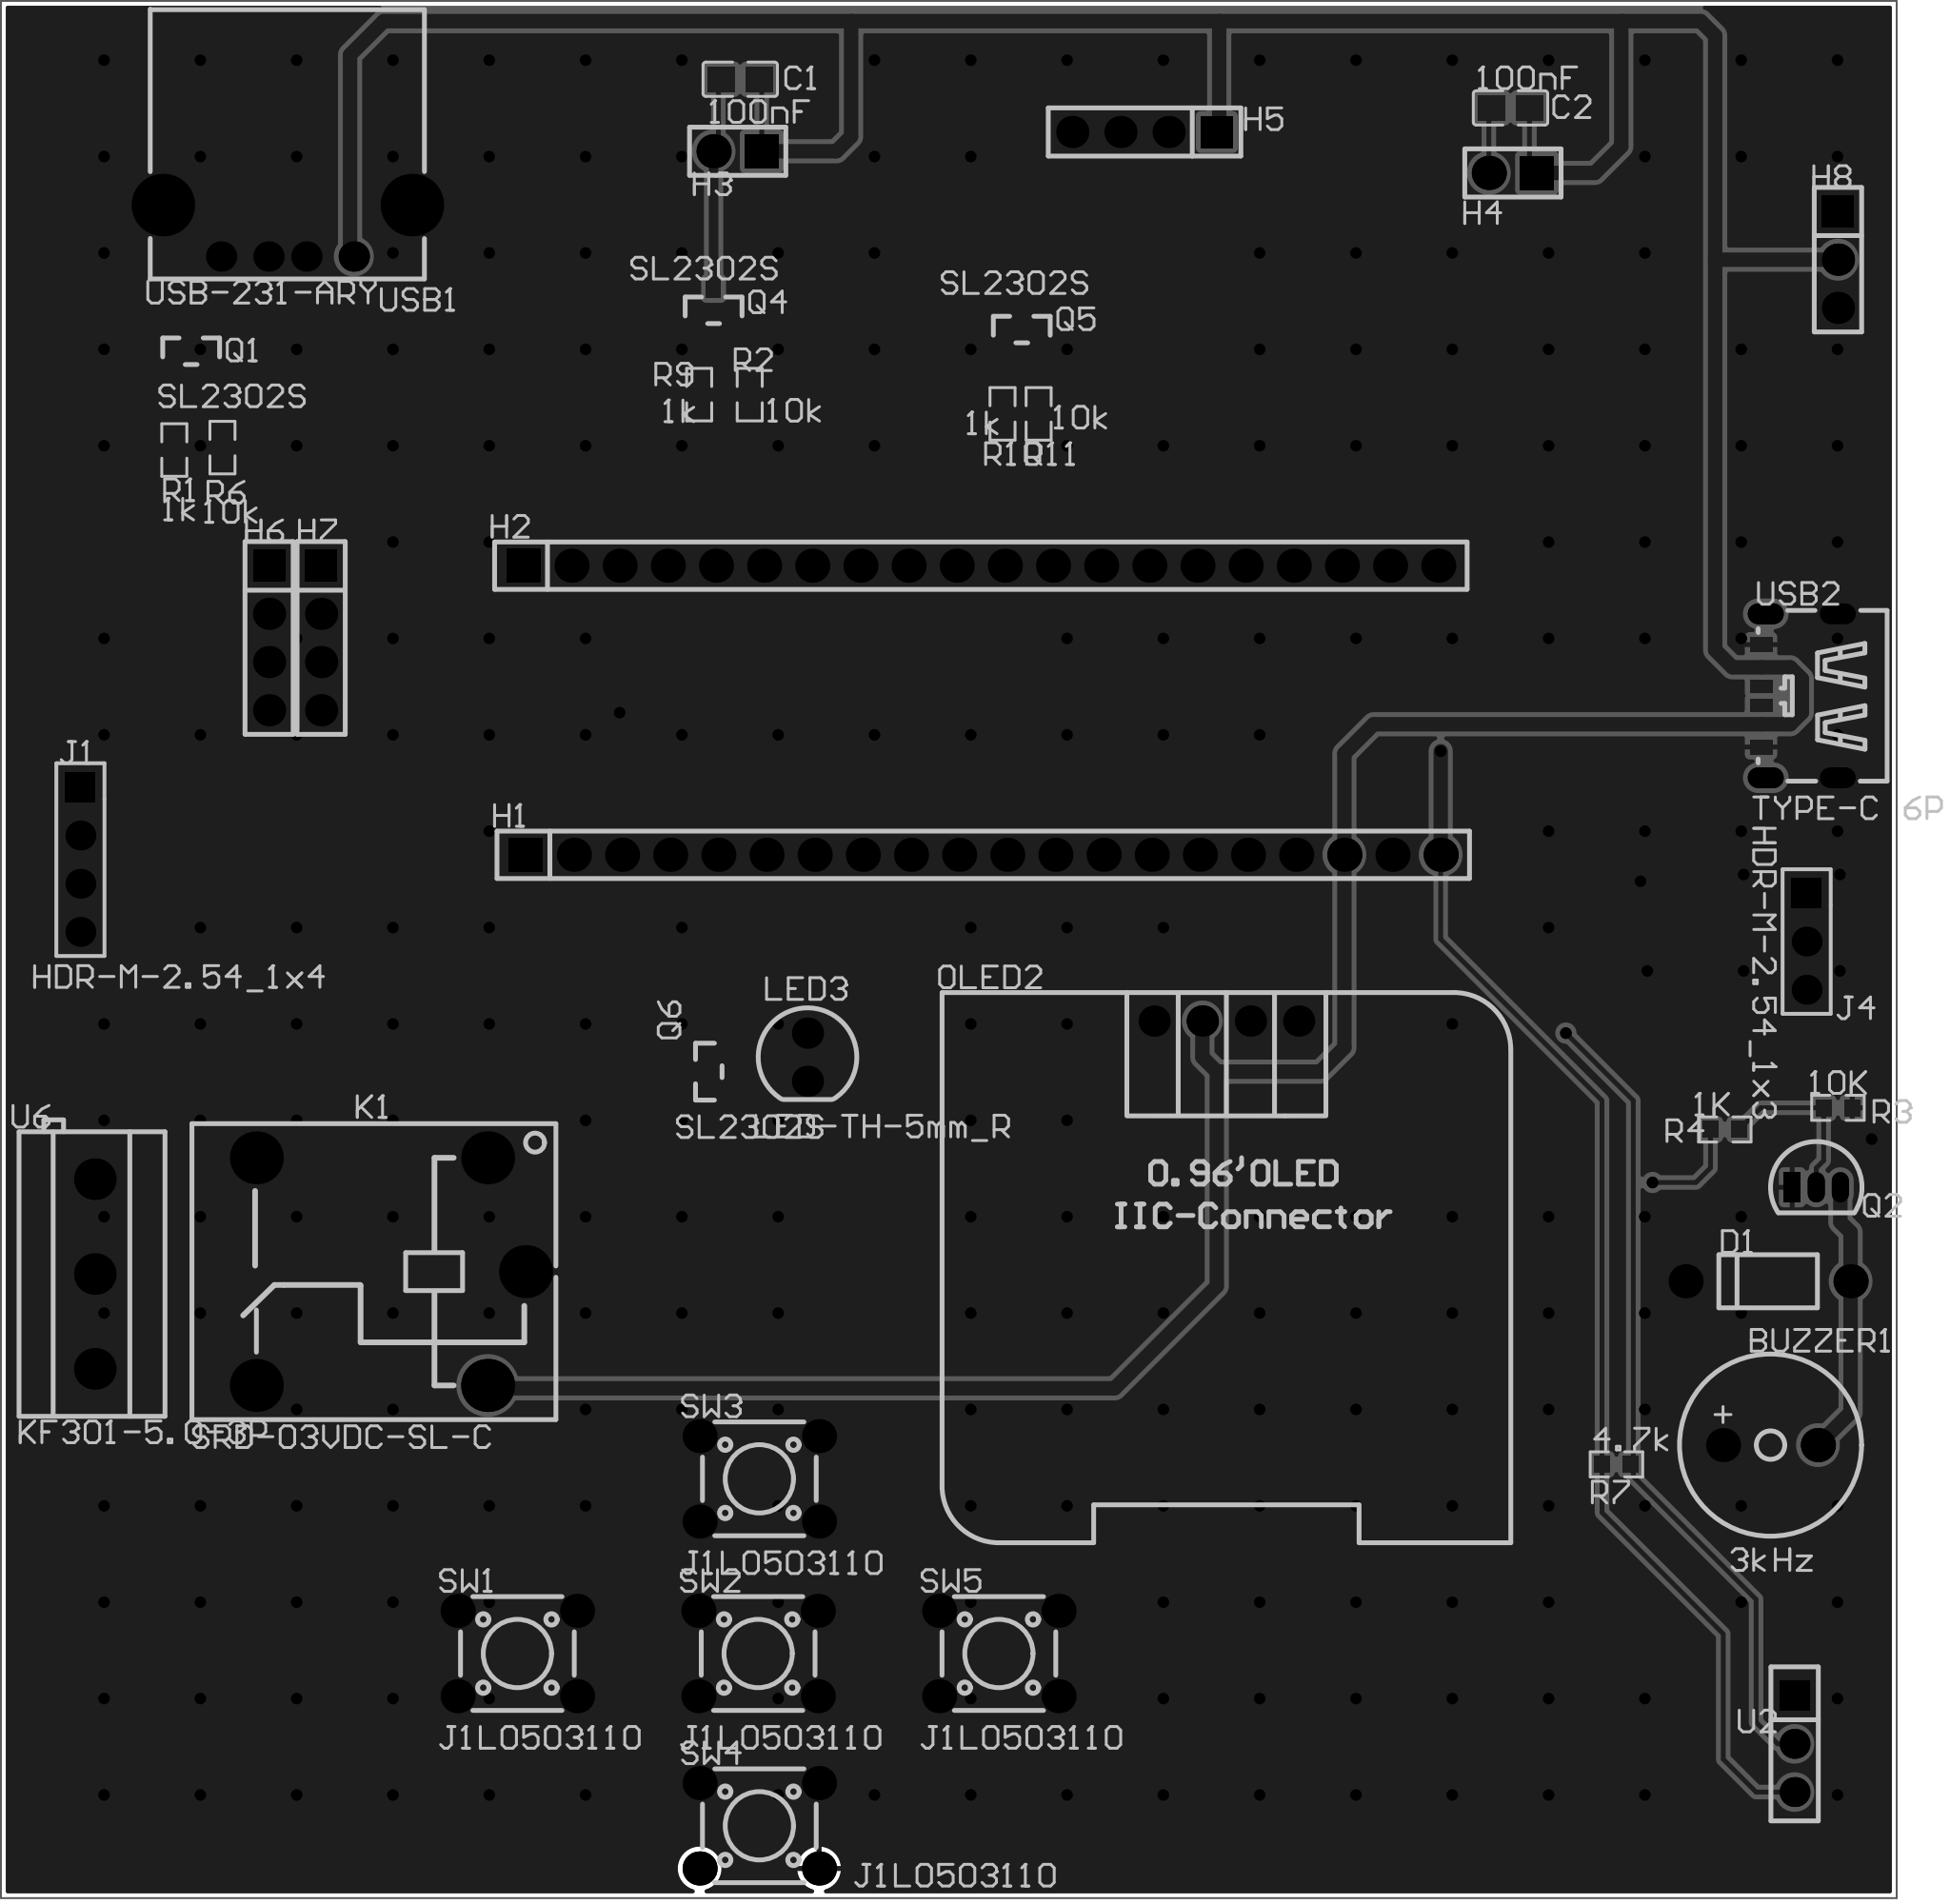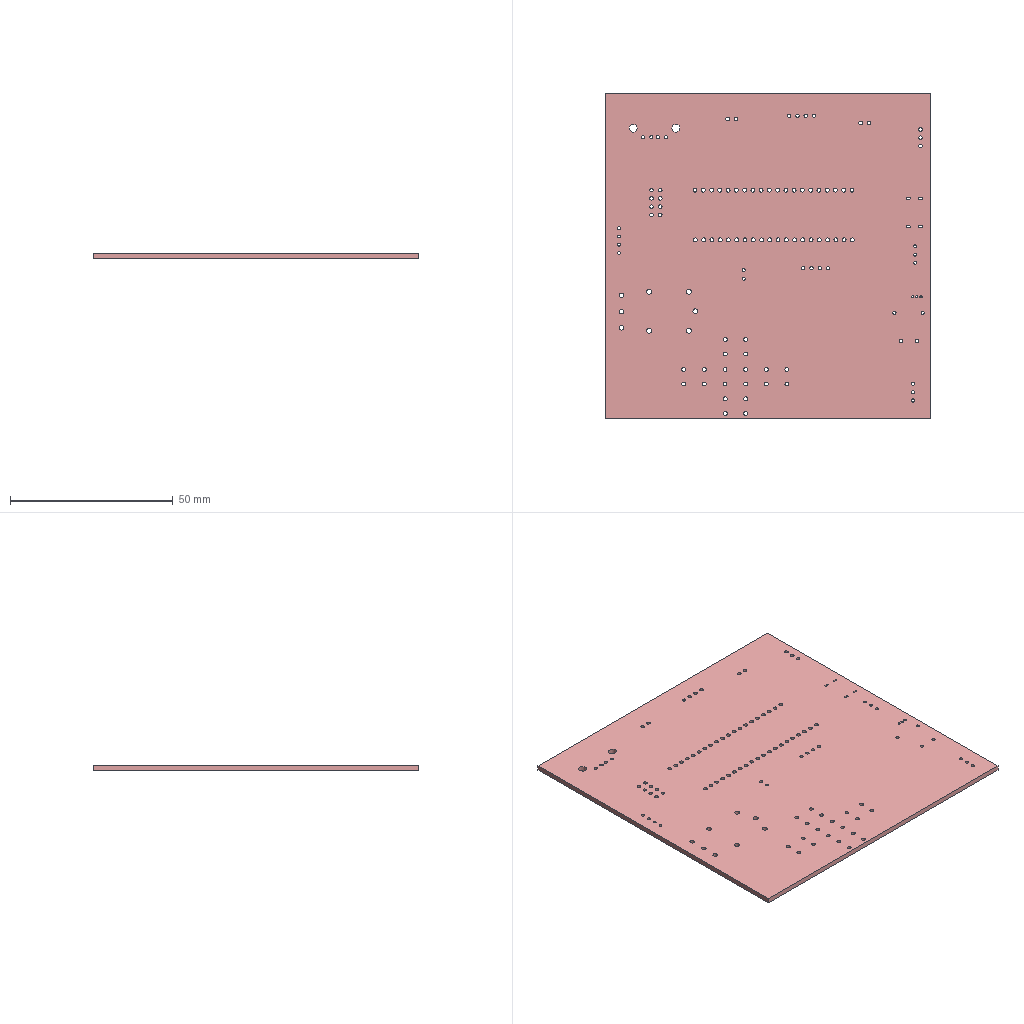Circuit board layout | Altium Designer | box 100 x 100 x 1.6 mm
Layer stack:
# Altium Designer layer stack of  (unit mm; dielectric type: 0 none, 1 core, 2 prepreg, 3 surface material)
index,name,kind,layer,copper_thickness_mm,dielectric_type,dielectric_thickness_mm,dielectric_material,dielectric_constant
0,Top Paste Mask Layer,other,,,,,,
1,Top Silkscreen Layer,other,,,,,,
2,Top Solder Mask Layer,dielectric,,,3,0.01,,3.3
3,Top Layer,copper,Top Layer,0.035,,,,
4,Dielectric1,dielectric,,,3,1.51,FR4,4.5
5,Bottom Layer,copper,Bottom Layer,0.035,,,,
6,Bottom Solder Mask Layer,dielectric,,,3,0.01,,3.3
7,Bottom Silkscreen Layer,other,,,,,,
8,Bottom Paste Mask Layer,other,,,,,,
# drill layer pairs: low layer,high layer
drill_pair,Top Layer,Bottom Layer
Part placement:
Designator,Comment,Layer,Footprint,Center-X(mm),Center-Y(mm),Rotation
BUZZER1,3kHz,TopLayer,BUZ-TH_BD9.6-P5.00-D0.7-FD,181.864,107.188,0
H1,,TopLayer,HDR-TH_20P-P2.54-V-F,140.335,138.303,0
H2,,TopLayer,HDR-TH_20P-P2.54-V-F,140.208,153.543,0
H3,,TopLayer,HDR-TH_2P-P2.54-V-M-1,127.381,175.387,180
H4,,TopLayer,HDR-TH_2P-P2.54-V-M-1,168.275,174.244,180
H5,,TopLayer,HDR-TH_4P-P2.54-V-M,148.844,176.403,180
H6,,TopLayer,HDR-TH_4P-P2.54-V-M,102.663,149.733,270
H7,,TopLayer,HDR-TH_4P-P2.54-V-M,105.41,149.733,270
H8,,TopLayer,HDR-TH_3P-P2.54-V-M,185.42,169.672,270
J1,HDR-M-2.54_1x4,TopLayer,HDR-M-2.54_1X4,92.71,138.049,270
J4,HDR-M-2.54_1x3,TopLayer,HDR-M-2.54_1X3,183.769,133.731,270
K1,SRD-03VDC-SL-C,TopLayer,RELAY-TH_SRD-XXVDC-XL-C,109.093,116.332,180
LED3,LED-TH-5mm_R,TopLayer,LED-TH_BD5.0_RED,131.064,127.635,0
OLED2,,TopLayer,0.96OLED_4P,153.162,129.54,0
Q1,SL2302S,TopLayer,SOT-23_L2.9-W1.3-P1.90-LS2.4-BR,98.552,164.846,270
Q4,SL2302S,TopLayer,SOT-23_L2.9-W1.3-P1.90-LS2.4-BR,126.111,167.005,270
Q5,SL2302S,TopLayer,SOT-23_L2.9-W1.3-P1.90-LS2.4-BR,142.367,165.989,270
Q6,SL2302S,TopLayer,SOT-23_L2.9-W1.3-P1.90-LS2.4-BR,125.857,126.873,0
R1,1k,TopLayer,R0603,97.663,159.639,90
R6,10k,TopLayer,R0603,100.203,159.766,90
R7,4.7k,TopLayer,R0603,173.736,106.172,180
R9,1k,TopLayer,R0603,125.349,162.56,90
R10,1k,TopLayer,R0603,141.351,161.544,90
R11,10k,TopLayer,R0603,143.256,161.544,90
SW1,J1L0503110,TopLayer,SW-TH_4P-L6.0-W6.0-P4.50-LS6.3,115.76,96.203,0
SW2,J1L0503110,TopLayer,SW-TH_4P-L6.0-W6.0-P4.50-LS6.3,128.46,96.203,0
SW3,J1L0503110,TopLayer,SW-TH_4P-L6.0-W6.0-P4.50-LS6.3,128.524,105.41,0
SW4,J1L0503110,TopLayer,SW-TH_4P-L6.0-W6.0-P4.50-LS6.3,128.524,87.122,0
SW5,J1L0503110,TopLayer,SW-TH_4P-L6.0-W6.0-P4.50-LS6.3,141.161,96.203,0
U6,KF301-5.0-3P,TopLayer,CONN-TH_3P-P5.00_KF301-5.0-3P,93.472,116.205,90
USB1,USB-231-ARY,TopLayer,USB-A-TH_USB-231-ARY,103.632,171.196,180
USB2,TYPE-C 6P,TopLayer,TYPE-C-SMD_TYPE-C-6P_1,183.388,146.685,90
C1,100nF,TopLayer,C0805,127.516,179.184,180
C2,100nF,TopLayer,C0805,168.148,177.673,180
R2,10k,TopLayer,R0603,128.016,162.56,90
D1,,TopLayer,DO_1N4007,181.737,115.824,0
Q2,,TopLayer,S8050_TO_92,184.277,120.777,0
R3,10K,TopLayer,R0603,185.42,124.968,180
R4,1K,TopLayer,R0603,179.451,123.825,180
U2,DS18B20+,TopLayer,HDR-TH_3P-P2.54-V-F,183.134,91.44,270
Pad and via stacks:
# Altium Designer via and pad stacks of  (unit mm). Each distinct definition once, with the count of objects using it.
# via: kind,start_layer,end_layer,hole_mm,diameter_mm,mode(0 simple;1 top-mid-bottom;2 full stack),diameter_per_layer,count,example_net
# pad: kind,layer,hole_mm,hole_type(0 round;1 square;2 slot),plating,top_size,top_shape(1 round;2 rect;3 octagon;9 rounded rect),mid_size,bottom_size,mode,footprint,size_per_layer,count,example
pad,Multi-Layer,1,0,plated,1.8x1.8,1,1.8x1.8,1.8x1.8,0,BUZ-TH_BD9.6-P5.00-D0.7-FD,,2,BUZZER1.2
pad,Multi-Layer,1.2,0,plated,1.8x1.8,2,1.8x1.8,1.8x1.8,0,HDR-TH_20P-P2.54-V-F,,2,H1.1
pad,Multi-Layer,1.2,0,plated,1.8x1.8,1,1.8x1.8,1.8x1.8,0,HDR-TH_20P-P2.54-V-F,,38,H1.2
pad,Multi-Layer,1.1,0,plated,1.8x1.8,1,1.8x1.8,1.8x1.8,0,HDR-TH_2P-P2.54-V-M-1,,2,H3.2
pad,Multi-Layer,1.1,0,plated,1.8x1.8,2,1.8x1.8,1.8x1.8,0,HDR-TH_2P-P2.54-V-M-1,,2,H3.1
pad,Multi-Layer,1.1,0,plated,1.7x1.7,2,1.7x1.7,1.7x1.7,0,HDR-TH_4P-P2.54-V-M,,3,H5.1
pad,Multi-Layer,1.1,0,plated,1.7x1.7,1,1.7x1.7,1.7x1.7,0,HDR-TH_4P-P2.54-V-M,,9,H5.2
pad,Multi-Layer,1.1,0,plated,1.7x1.7,2,1.7x1.7,1.7x1.7,0,HDR-TH_3P-P2.54-V-M,,1,H8.1
pad,Multi-Layer,1.1,0,plated,1.7x1.7,1,1.7x1.7,1.7x1.7,0,HDR-TH_3P-P2.54-V-M,,2,H8.2
pad,Multi-Layer,0.889,0,plated,1.575x1.575,2,1.575x1.575,1.575x1.575,0,HDR-M-2.54_1X4,,1,J1.1
pad,Multi-Layer,0.889,0,plated,1.575x1.575,1,1.575x1.575,1.575x1.575,0,HDR-M-2.54_1X4,,3,J1.2
pad,Multi-Layer,0.889,0,plated,1.575x1.575,1,1.575x1.575,1.575x1.575,0,HDR-M-2.54_1X3,,2,J4.3
pad,Multi-Layer,0.889,0,plated,1.575x1.575,2,1.575x1.575,1.575x1.575,0,HDR-M-2.54_1X3,,1,J4.1
pad,Multi-Layer,1.524,0,plated,2.794x2.794,1,2.794x2.794,2.794x2.794,0,RELAY-TH_SRD-XXVDC-XL-C,,5,K1.2
pad,Multi-Layer,0.9652,0,plated,1.651x1.651,1,1.651x1.651,1.651x1.651,0,LED-TH_BD5.0_RED,,2,LED3.1
pad,Multi-Layer,1,0,plated,1.65x1.65,1,1.65x1.65,1.65x1.65,0,0.96OLED_4P,,4,OLED2.4
pad,Multi-Layer,1.2,0,plated,1.8x1.8,1,1.8x1.8,1.8x1.8,0,SW-TH_4P-L6.0-W6.0-P4.50-LS6.3,,20,SW1.1
pad,Multi-Layer,1.4,0,plated,2.2x2.2,1,2.2x2.2,2.2x2.2,0,CONN-TH_3P-P5.00_KF301-5.0-3P,,3,U6.1
pad,Multi-Layer,1,0,plated,1.6x1.6,1,1.6x1.6,1.6x1.6,0,USB-A-TH_USB-231-ARY,,4,USB1.1
pad,Multi-Layer,2.5,0,plated,3.3x3.3,1,3.3x3.3,3.3x3.3,0,USB-A-TH_USB-231-ARY,,2,USB1.5
pad,Multi-Layer,0.6,2,plated,1.1x1.9,1,1.1x1.9,1.1x1.9,0,TYPE-C-SMD_TYPE-C-6P_1,,4,USB2.7
pad,Multi-Layer,1,0,plated,1.8x1.8,1,1.8x1.8,1.8x1.8,0,DO_1N4007,,2,D1.1
pad,Multi-Layer,0.701,0,plated,0.8992x1.6,2,0.8992x1.6,0.8992x1.6,0,S8050_TO_92,,1,Q2.1
pad,Multi-Layer,0.701,0,plated,0.8992x1.6,1,0.8992x1.6,0.8992x1.6,0,S8050_TO_92,,2,Q2.2
pad,Multi-Layer,1.02,0,plated,1.575x1.575,1,1.575x1.575,1.575x1.575,0,HDR-TH_3P-P2.54-V-F,,2,U2.3
pad,Multi-Layer,1.02,0,plated,1.575x1.575,2,1.575x1.575,1.575x1.575,0,HDR-TH_3P-P2.54-V-F,,1,U2.1
pad,Top Layer,0,0,plated,1x0.8,2,1x0.8,1x0.8,0,SOT-23_L2.9-W1.3-P1.90-LS2.4-BR,,12,Q1.2
pad,Top Layer,0,0,plated,0.8065x0.864,2,0.8065x0.864,0.8065x0.864,0,R0603,,18,R1.2
pad,Top Layer,0,0,plated,0.8x1.2,2,0.8x1.2,0.8x1.2,0,TYPE-C-SMD_TYPE-C-6P_1,,2,USB2.B12
pad,Top Layer,0,0,plated,0.7x1.2,2,0.7x1.2,0.7x1.2,0,TYPE-C-SMD_TYPE-C-6P_1,,4,USB2.B9
pad,Top Layer,0,0,plated,1.41x1.35,2,1.41x1.35,1.41x1.35,0,C0805,,4,C1.2
via,Top Layer,Bottom Layer,0.3048,0.61,0,,267,$1N30
Copper pours:
name,layer,net,type(0 solid;1 hatched;2 none)
Top Layer-GND,Top Layer,GND,0
Bottom Layer-GND,Bottom Layer,GND,0
Design rules, without the lines most boards share:
# Altium Designer design rules of  (exported by Altium Designer, unit mm)
# columns: name | kind | enabled | priority | scope1 | scope2 | descriptor | typed fields (field=value)
Copper_copperRegion_copperThickness1oz | 0 | disabled | 4 | All | All | Clearance Constraint (Gap=5.984mil) (Disabled)(All),(All) | gap=0.152
Copper_copperRegion_copperThickness1oz_1 | 63 | disabled | 4 | All | All | Board Clearance Constraint (Gap=0mil) (Disabled)(All) |
Copper_copperRegion_Copper_copperRegion | 0 | disabled | 5 | All | All | Clearance Constraint (Gap=5.984mil) (Disabled)(All),(All) | gap=0.152
Copper_copperRegion_Copper_copperRegion_1 | 63 | disabled | 5 | All | All | Board Clearance Constraint (Gap=0mil) (Disabled)(All) |
copperThickness1oz | 0 | enabled | 6 | All | All | Clearance Constraint (Gap=5.984mil) (All),(All) | gap=0.152
copperThickness1oz_1 | 63 | enabled | 6 | All | All | Board Clearance Constraint (Gap=0mil) (All) |
copperRegion_copperThickness1oz | 20 | disabled | 1 | All | All | Polygon Connect Rule(Relief Connect )(Conductor Width=10mil) (Relief Angle=90 Angle) (Entries=4) (Air Gap Width=10mil) (Disabled)(All),(All) | connect_style(0=relief,1=direct,2=none)=0 relief_conductor_width=0.254 relief_entries=4
copperRegion_Copper_copperRegion | 20 | disabled | 2 | All | All | Polygon Connect Rule(Relief Connect )(Conductor Width=10mil) (Relief Angle=90 Angle) (Entries=4) (Air Gap Width=10mil) (Disabled)(All),(All) | connect_style(0=relief,1=direct,2=none)=0 relief_conductor_width=0.254 relief_entries=4
copperRegion | 20 | enabled | 3 | All | All | Polygon Connect Rule(Relief Connect )(Conductor Width=10mil) (Relief Angle=90 Angle) (Entries=4) (Air Gap Width=10mil) (All),(All) | connect_style(0=relief,1=direct,2=none)=0 relief_conductor_width=0.254 relief_entries=4